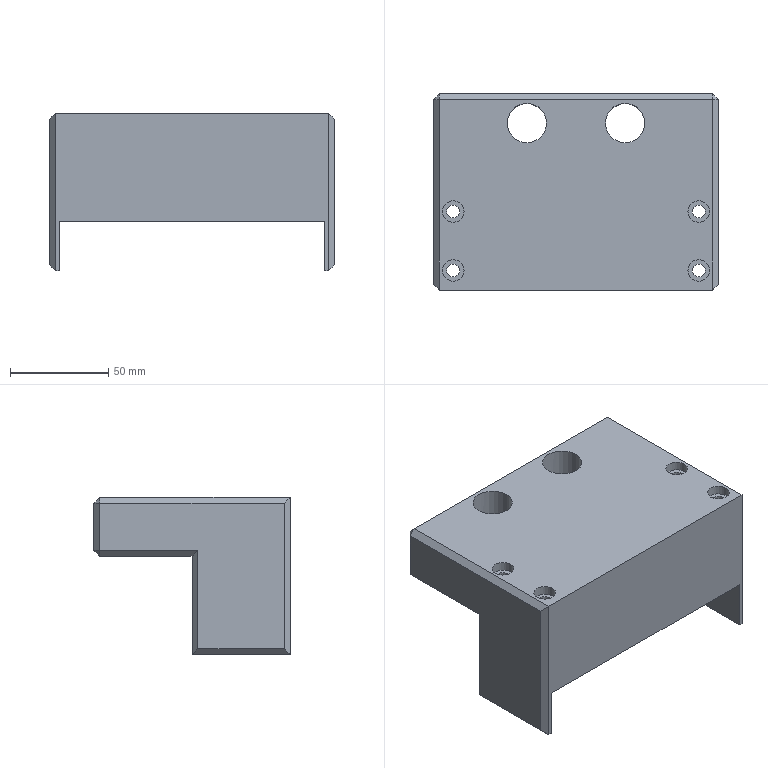NC program | NX | posted with a generic post | part box 145 x 100 x 80 mm
Lines 1 to 550 of 2025:
N10 G17 G21 G94 G90
(FLOOR_WALL_2 , TOOL : D63)
N12 T01 M6
N14 G54
N16 G17 G0 G90 X-109.603 Y-18.5 B0. C0. S6500 M3
N18 G43 Z30. H1
N20 Z0.502
N22 G94 G1 Z-0.998 F1000.
N24 G3 X-104.147 Y-21.65 R6.3
N26 G1 X104.147 F1500.
N28 G3 X109.603 Y-18.5 R6.3
N30 G1 Z0.502
N32 G0 Z30.
N34 X-109.603
N36 Z-0.496
N38 G1 Z-1.996 F1000.
N40 G3 X-104.147 Y-21.65 R6.3
N42 G1 X104.147 F1500.
N44 G3 X109.603 Y-18.5 R6.3
N46 G1 Z-0.496
N48 G0 Z30.
N50 X-109.603
N52 Z-1.494
N54 G1 Z-2.994 F1000.
N56 G3 X-104.147 Y-21.65 R6.3
N58 G1 X104.147 F1500.
N60 G3 X109.603 Y-18.5 R6.3
N62 G1 Z-1.494
N64 G0 Z30.
N66 X-109.603
N68 Z-2.492
N70 G1 Z-3.992 F1000.
N72 G3 X-104.147 Y-21.65 R6.3
N74 G1 X104.147 F1500.
N76 G3 X109.603 Y-18.5 R6.3
N78 G1 Z-2.492
N80 G0 Z30.
N82 X-109.603
N84 Z-3.49
N86 G1 Z-4.99 F1000.
N88 G3 X-104.147 Y-21.65 R6.3
N90 G1 X104.147 F1500.
N92 G3 X109.603 Y-18.5 R6.3
N94 G1 Z-3.49
N96 G0 Z30.
N98 X-109.603
N100 Z-4.488
N102 G1 Z-5.988 F1000.
N104 G3 X-104.147 Y-21.65 R6.3
N106 G1 X104.147 F1500.
N108 G3 X109.603 Y-18.5 R6.3
N110 G1 Z-4.488
N112 G0 Z30.
N114 X-109.603
N116 Z-5.486
N118 G1 Z-6.986 F1000.
N120 G3 X-104.147 Y-21.65 R6.3
N122 G1 X104.147 F1500.
N124 G3 X109.603 Y-18.5 R6.3
N126 G1 Z-5.486
N128 G0 Z30.
N130 X-109.603
N132 Z-6.484
N134 G1 Z-7.984 F1000.
N136 G3 X-104.147 Y-21.65 R6.3
N138 G1 X104.147 F1500.
N140 G3 X109.603 Y-18.5 R6.3
N142 G1 Z-6.484
N144 G0 Z30.
N146 X-109.603
N148 Z-7.482
N150 G1 Z-8.982 F1000.
N152 G3 X-104.147 Y-21.65 R6.3
N154 G1 X104.147 F1500.
N156 G3 X109.603 Y-18.5 R6.3
N158 G1 Z-7.482
N160 G0 Z30.
N162 X-109.603
N164 Z-8.48
N166 G1 Z-9.98 F1000.
N168 G3 X-104.147 Y-21.65 R6.3
N170 G1 X104.147 F1500.
N172 G3 X109.603 Y-18.5 R6.3
N174 G1 Z-8.48
N176 G0 Z30.
N178 X-109.603
N180 Z-9.478
N182 G1 Z-10.978 F1000.
N184 G3 X-104.147 Y-21.65 R6.3
N186 G1 X104.147 F1500.
N188 G3 X109.603 Y-18.5 R6.3
N190 G1 Z-9.478
N192 G0 Z30.
N194 X-109.603
N196 Z-10.476
N198 G1 Z-11.976 F1000.
N200 G3 X-104.147 Y-21.65 R6.3
N202 G1 X104.147 F1500.
N204 G3 X109.603 Y-18.5 R6.3
N206 G1 Z-10.476
N208 G0 Z30.
N210 X-109.603
N212 Z-11.474
N214 G1 Z-12.974 F1000.
N216 G3 X-104.147 Y-21.65 R6.3
N218 G1 X104.147 F1500.
N220 G3 X109.603 Y-18.5 R6.3
N222 G1 Z-11.474
N224 G0 Z30.
N226 X-109.603
N228 Z-12.472
N230 G1 Z-13.972 F1000.
N232 G3 X-104.147 Y-21.65 R6.3
N234 G1 X104.147 F1500.
N236 G3 X109.603 Y-18.5 R6.3
N238 G1 Z-12.472
N240 G0 Z30.
N242 X-109.603
N244 Z-13.47
N246 G1 Z-14.97 F1000.
N248 G3 X-104.147 Y-21.65 R6.3
N250 G1 X104.147 F1500.
N252 G3 X109.603 Y-18.5 R6.3
N254 G1 Z-13.47
N256 G0 Z30.
N258 X-109.603
N260 Z-14.468
N262 G1 Z-15.968 F1000.
N264 G3 X-104.147 Y-21.65 R6.3
N266 G1 X104.147 F1500.
N268 G3 X109.603 Y-18.5 R6.3
N270 G1 Z-14.468
N272 G0 Z30.
N274 X-109.603
N276 Z-15.466
N278 G1 Z-16.966 F1000.
N280 G3 X-104.147 Y-21.65 R6.3
N282 G1 X104.147 F1500.
N284 G3 X109.603 Y-18.5 R6.3
N286 G1 Z-15.466
N288 G0 Z30.
N290 X-109.603
N292 Z-16.464
N294 G1 Z-17.964 F1000.
N296 G3 X-104.147 Y-21.65 R6.3
N298 G1 X104.147 F1500.
N300 G3 X109.603 Y-18.5 R6.3
N302 G1 Z-16.464
N304 G0 Z30.
N306 X-109.603
N308 Z-17.462
N310 G1 Z-18.962 F1000.
N312 G3 X-104.147 Y-21.65 R6.3
N314 G1 X104.147 F1500.
N316 G3 X109.603 Y-18.5 R6.3
N318 G1 Z-17.462
N320 G0 Z30.
N322 X-109.603
N324 Z-18.46
N326 G1 Z-19.96 F1000.
N328 G3 X-104.147 Y-21.65 R6.3
N330 G1 X104.147 F1500.
N332 G3 X109.603 Y-18.5 R6.3
N334 G1 Z-18.46
N336 G0 Z30.
N338 X-109.603
N340 Z-19.458
N342 G1 Z-20.958 F1000.
N344 G3 X-104.147 Y-21.65 R6.3
N346 G1 X104.147 F1500.
N348 G3 X109.603 Y-18.5 R6.3
N350 G1 Z-19.458
N352 G0 Z30.
N354 X-109.603
N356 Z-20.456
N358 G1 Z-21.956 F1000.
N360 G3 X-104.147 Y-21.65 R6.3
N362 G1 X104.147 F1500.
N364 G3 X109.603 Y-18.5 R6.3
N366 G1 Z-20.456
N368 G0 Z30.
N370 X-109.603
N372 Z-21.454
N374 G1 Z-22.954 F1000.
N376 G3 X-104.147 Y-21.65 R6.3
N378 G1 X104.147 F1500.
N380 G3 X109.603 Y-18.5 R6.3
N382 G1 Z-21.454
N384 G0 Z30.
N386 X-109.603
N388 Z-22.452
N390 G1 Z-23.952 F1000.
N392 G3 X-104.147 Y-21.65 R6.3
N394 G1 X104.147 F1500.
N396 G3 X109.603 Y-18.5 R6.3
N398 G1 Z-22.452
N400 G0 Z30.
N402 X-109.603
N404 Z-23.45
N406 G1 Z-24.95 F1000.
N408 G3 X-104.147 Y-21.65 R6.3
N410 G1 X104.147 F1500.
N412 G3 X109.603 Y-18.5 R6.3
N414 G1 Z-23.45
N416 G0 Z30.
N418 X-109.603
N420 Z-24.448
N422 G1 Z-25.948 F1000.
N424 G3 X-104.147 Y-21.65 R6.3
N426 G1 X104.147 F1500.
N428 G3 X109.603 Y-18.5 R6.3
N430 G1 Z-24.448
N432 G0 Z30.
N434 X-109.603
N436 Z-25.446
N438 G1 Z-26.946 F1000.
N440 G3 X-104.147 Y-21.65 R6.3
N442 G1 X104.147 F1500.
N444 G3 X109.603 Y-18.5 R6.3
N446 G1 Z-25.446
N448 G0 Z30.
N450 X-109.603
N452 Z-26.444
N454 G1 Z-27.944 F1000.
N456 G3 X-104.147 Y-21.65 R6.3
N458 G1 X104.147 F1500.
N460 G3 X109.603 Y-18.5 R6.3
N462 G1 Z-26.444
N464 G0 Z30.
N466 X-109.603
N468 Z-27.442
N470 G1 Z-28.942 F1000.
N472 G3 X-104.147 Y-21.65 R6.3
N474 G1 X104.147 F1500.
N476 G3 X109.603 Y-18.5 R6.3
N478 G1 Z-27.442
N480 G0 Z30.
N482 X-109.603
N484 Z-28.44
N486 G1 Z-29.94 F1000.
N488 G3 X-104.147 Y-21.65 R6.3
N490 G1 X104.147 F1500.
N492 G3 X109.603 Y-18.5 R6.3
N494 G1 Z-28.44
N496 G0 Z30.
N498 X-109.603
N500 Z-29.438
N502 G1 Z-30.938 F1000.
N504 G3 X-104.147 Y-21.65 R6.3
N506 G1 X104.147 F1500.
N508 G3 X109.603 Y-18.5 R6.3
N510 G1 Z-29.438
N512 G0 Z30.
N514 X-109.603
N516 Z-30.436
N518 G1 Z-31.936 F1000.
N520 G3 X-104.147 Y-21.65 R6.3
N522 G1 X104.147 F1500.
N524 G3 X109.603 Y-18.5 R6.3
N526 G1 Z-30.436
N528 G0 Z30.
N530 X-109.603
N532 Z-31.434
N534 G1 Z-32.934 F1000.
N536 G3 X-104.147 Y-21.65 R6.3
N538 G1 X104.147 F1500.
N540 G3 X109.603 Y-18.5 R6.3
N542 G1 Z-31.434
N544 G0 Z30.
N546 X-109.603
N548 Z-32.432
N550 G1 Z-33.932 F1000.
N552 G3 X-104.147 Y-21.65 R6.3
N554 G1 X104.147 F1500.
N556 G3 X109.603 Y-18.5 R6.3
N558 G1 Z-32.432
N560 G0 Z30.
N562 X-109.603
N564 Z-33.43
N566 G1 Z-34.93 F1000.
N568 G3 X-104.147 Y-21.65 R6.3
N570 G1 X104.147 F1500.
N572 G3 X109.603 Y-18.5 R6.3
N574 G1 Z-33.43
N576 G0 Z30.
N578 X-109.603
N580 Z-34.428
N582 G1 Z-35.928 F1000.
N584 G3 X-104.147 Y-21.65 R6.3
N586 G1 X104.147 F1500.
N588 G3 X109.603 Y-18.5 R6.3
N590 G1 Z-34.428
N592 G0 Z30.
N594 X-109.603
N596 Z-35.426
N598 G1 Z-36.926 F1000.
N600 G3 X-104.147 Y-21.65 R6.3
N602 G1 X104.147 F1500.
N604 G3 X109.603 Y-18.5 R6.3
N606 G1 Z-35.426
N608 G0 Z30.
N610 X-109.603
N612 Z-36.424
N614 G1 Z-37.924 F1000.
N616 G3 X-104.147 Y-21.65 R6.3
N618 G1 X104.147 F1500.
N620 G3 X109.603 Y-18.5 R6.3
N622 G1 Z-36.424
N624 G0 Z30.
N626 X-109.603
N628 Z-37.422
N630 G1 Z-38.922 F1000.
N632 G3 X-104.147 Y-21.65 R6.3
N634 G1 X104.147 F1500.
N636 G3 X109.603 Y-18.5 R6.3
N638 G1 Z-37.422
N640 G0 Z30.
N642 X-109.603
N644 Z-38.42
N646 G1 Z-39.92 F1000.
N648 G3 X-104.147 Y-21.65 R6.3
N650 G1 X104.147 F1500.
N652 G3 X109.603 Y-18.5 R6.3
N654 G1 Z-38.42
N656 G0 Z30.
N658 X-109.603
N660 Z-39.418
N662 G1 Z-40.918 F1000.
N664 G3 X-104.147 Y-21.65 R6.3
N666 G1 X104.147 F1500.
N668 G3 X109.603 Y-18.5 R6.3
N670 G1 Z-39.418
N672 G0 Z30.
N674 X-109.603
N676 Z-40.416
N678 G1 Z-41.916 F1000.
N680 G3 X-104.147 Y-21.65 R6.3
N682 G1 X104.147 F1500.
N684 G3 X109.603 Y-18.5 R6.3
N686 G1 Z-40.416
N688 G0 Z30.
N690 X-109.603
N692 Z-41.414
N694 G1 Z-42.914 F1000.
N696 G3 X-104.147 Y-21.65 R6.3
N698 G1 X104.147 F1500.
N700 G3 X109.603 Y-18.5 R6.3
N702 G1 Z-41.414
N704 G0 Z30.
N706 X-109.603
N708 Z-42.412
N710 G1 Z-43.912 F1000.
N712 G3 X-104.147 Y-21.65 R6.3
N714 G1 X104.147 F1500.
N716 G3 X109.603 Y-18.5 R6.3
N718 G1 Z-42.412
N720 G0 Z30.
N722 X-109.603
N724 Z-43.41
N726 G1 Z-44.91 F1000.
N728 G3 X-104.147 Y-21.65 R6.3
N730 G1 X104.147 F1500.
N732 G3 X109.603 Y-18.5 R6.3
N734 G1 Z-43.41
N736 G0 Z30.
N738 X-109.603
N740 Z-44.408
N742 G1 Z-45.908 F1000.
N744 G3 X-104.147 Y-21.65 R6.3
N746 G1 X104.147 F1500.
N748 G3 X109.603 Y-18.5 R6.3
N750 G1 Z-44.408
N752 G0 Z30.
N754 X-109.603
N756 Z-45.406
N758 G1 Z-46.906 F1000.
N760 G3 X-104.147 Y-21.65 R6.3
N762 G1 X104.147 F1500.
N764 G3 X109.603 Y-18.5 R6.3
N766 G1 Z-45.406
N768 G0 Z30.
N770 X-109.603
N772 Z-46.404
N774 G1 Z-47.904 F1000.
N776 G3 X-104.147 Y-21.65 R6.3
N778 G1 X104.147 F1500.
N780 G3 X109.603 Y-18.5 R6.3
N782 G1 Z-46.404
N784 G0 Z30.
N786 X-109.603
N788 Z-47.402
N790 G1 Z-48.902 F1000.
N792 G3 X-104.147 Y-21.65 R6.3
N794 G1 X104.147 F1500.
N796 G3 X109.603 Y-18.5 R6.3
N798 G1 Z-47.402
N800 G0 Z30.
N802 X-109.603
N804 Z-48.4
N806 G1 Z-49.9 F1000.
N808 G3 X-104.147 Y-21.65 R6.3
N810 G1 X104.147 F1500.
N812 G3 X109.603 Y-18.5 R6.3
N814 G1 Z-48.4
N816 G0 Z30.
N818 M5
(FLOOR_WALL_1_COPY_COPY_COPY_COPY , TOOL : D10JING)
N820 T04 M6
N822 G54
N824 G17 G0 G90 X79. Y11.043 B0. C0. S7500 M3
N826 G43 Z30. H4
N828 Z-8.48
N830 G94 G1 Z-9.98 F1250.
N832 X78.465 Y11.187
N834 G3 X77.499 Y10.928 R1.
N836 G1 X71.571 Y5.
N838 X-71.571
N840 X-77.499 Y10.928
N842 G3 X-78.465 Y11.187 R1.
N844 G1 X-79. Y11.043
N846 Z-8.48
N848 G0 Z30.
N850 X79.
N852 Z-18.46
N854 G1 Z-19.96
N856 X78.465 Y11.187
N858 G3 X77.499 Y10.928 R1.
N860 G1 X71.571 Y5.
N862 X-71.571
N864 X-77.499 Y10.928
N866 G3 X-78.465 Y11.187 R1.
N868 G1 X-79. Y11.043
N870 Z-18.46
N872 G0 Z30.
N874 X79.
N876 Z-28.44
N878 G1 Z-29.94
N880 X78.465 Y11.187
N882 G3 X77.499 Y10.928 R1.
N884 G1 X71.571 Y5.
N886 X-71.571
N888 X-77.499 Y10.928
N890 G3 X-78.465 Y11.187 R1.
N892 G1 X-79. Y11.043
N894 Z-28.44
N896 G0 Z30.
N898 X79.
N900 Z-38.42
N902 G1 Z-39.92
N904 X78.465 Y11.187
N906 G3 X77.499 Y10.928 R1.
N908 G1 X71.571 Y5.
N910 X-71.571
N912 X-77.499 Y10.928
N914 G3 X-78.465 Y11.187 R1.
N916 G1 X-79. Y11.043
N918 Z-38.42
N920 G0 Z30.
N922 X79.
N924 Z-48.4
N926 G1 Z-49.9
N928 X78.465 Y11.187
N930 G3 X77.499 Y10.928 R1.
N932 G1 X71.571 Y5.
N934 X-71.571
N936 X-77.499 Y10.928
N938 G3 X-78.465 Y11.187 R1.
N940 G1 X-79. Y11.043
N942 Z-48.4
N944 G0 Z30.
(FLOOR_WALL_1_COPY_COPY_COPY , TOOL : D10JING)
N946 X-78.999 Y6.819
N948 Z-48.5
N950 G1 Z-50.
N952 X-78.365 Y5.721
N954 G3 X-77.499 Y5.221 R1.
N956 G1 X-72.499
N958 X-71.925 Y4.646
N960 G3 X-71.571 Y4.5 R0.5
N962 G1 X71.571
N964 G3 X71.925 Y4.646 R0.5
N966 G1 X72.499 Y5.221
N968 X77.499
N970 Y0.641
N972 X-77.499
N974 Y-3.939
N976 X77.499
N978 Y-8.519
N980 X-77.499
N982 Y-13.099
N984 X77.499
N986 Y-17.679
N988 X-77.499
N990 Y-22.259
N992 X77.499
N994 Y-26.839
N996 X-77.499
N998 Y-31.419
N1000 X77.499
N1002 Y-35.999
N1004 X-77.499
N1006 G2 X-78.365 Y-35.499 R1.
N1008 G1 X-78.999 Y-34.401
N1010 Z-48.5
N1012 G0 Z30.
N1014 X79. Y11.043
N1016 Z-48.5
N1018 G1 Z-50.
N1020 X78.465 Y11.187
N1022 G3 X77.499 Y10.928 R1.
N1024 G1 X71.571 Y5.
N1026 X-71.571
N1028 X-77.499 Y10.928
N1030 G3 X-78.465 Y11.187 R1.
N1032 G1 X-79. Y11.043
N1034 Z-48.5
N1036 G0 Z30.
N1038 M5
(DRILLING_COPY_2_COPY , TOOL : D8A45)
N1040 T06 M6
N1042 G54
N1044 G17 G0 G90 X-25. Y25. B0. C0. S3000 M3
N1046 G43 Z30. H6
N1048 G94 G81 G98 Z-3. F150. R3.
N1050 X25.
N1052 G80
N1054 G0 X25. Y25. Z30.
N1056 M5
(DRILLING_COPY_COPY_COPY_COPY_1_COPY_COPY_1 , TOOL : 5.0ZT)
N1058 T14 M6
N1060 G54
N1062 G17 G0 G90 X-25. Y25. B0. C0. S2000 M3
N1064 G43 Z30. H14
N1066 G94 G83 G98 Z-8.32 F150. Q2. R3.
N1068 X25.
N1070 G80
N1072 G0 X25. Y25. Z30.
N1074 M5